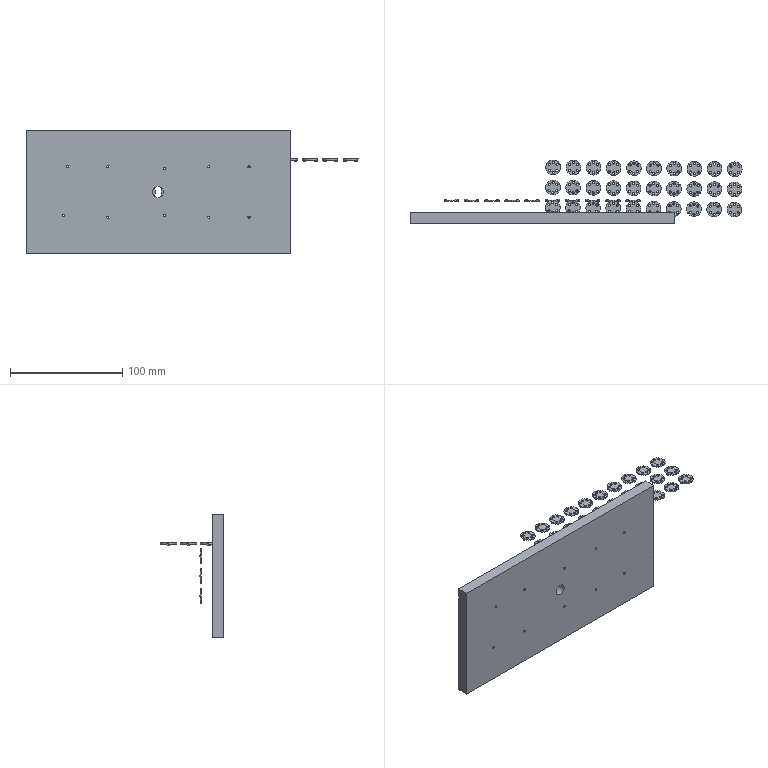NC program | NX | posted with a generic post | part box 296.27 x 56.878 x 110 mm
Lines 18830 to 20851 of 20851:
(DRILLING_COPY_1_COPY , TOOL : DJ-Ø3)
N37616 T04 M6
N37618 G17 G43 G0 G90 X84.467 Y15.117 Z1.5 B0. C0. S1500 H4 M3
N37620 G94 G81 G99 Z-2.1 F200. R0.
N37622 G0 Z4.
N37624 G81 X84.447 Y20.893 Z-2.1 R0.
N37626 G0 Z4.
N37628 G81 X81. Y22.5 Z-2.1 R0.
N37630 G0 Z4.
N37632 G81 X77.573 Y20.902 Z-2.1 R0.
N37634 G0 Z4.
N37636 G81 X77.553 Y15.107 Z-2.1 R0.
N37638 G0 Z4.
N37640 G81 X81. Y13.5 Z-2.1 R0.
N37642 G0 Z4.
N37644 G81 Y4.5 Z-2.1 R0.
N37646 G0 Z4.
N37648 G81 X77.573 Y2.902 Z-2.1 R0.
N37650 G0 Z4.
N37652 G81 X84.447 Y2.893 Z-2.1 R0.
N37654 G0 Z4.
N37656 G81 X84.467 Y-2.883 Z-2.1 R0.
N37658 G0 Z4.
N37660 G81 X81. Y-4.5 Z-2.1 R0.
N37662 G0 Z4.
N37664 G81 Y-13.5 Z-2.1 R0.
N37666 G0 Z4.
N37668 G81 X84.447 Y-15.107 Z-2.1 R0.
N37670 G0 Z4.
N37672 G81 X84.467 Y-20.883 Z-2.1 R0.
N37674 G0 Z4.
N37676 G81 X81. Y-22.5 Z-2.1 R0.
N37678 G0 Z4.
N37680 G81 X77.553 Y-20.893 Z-2.1 R0.
N37682 G0 Z4.
N37684 G81 X77.573 Y-15.098 Z-2.1 R0.
N37686 G0 Z4.
N37688 G81 X77.553 Y-2.893 Z-2.1 R0.
N37690 G0 Z4.
N37692 G81 X66.467 Y-2.883 Z-2.1 R0.
N37694 G0 Z4.
N37696 G81 X63. Y-4.5 Z-2.1 R0.
N37698 G0 Z4.
N37700 G81 X59.553 Y-2.893 Z-2.1 R0.
N37702 G0 Z4.
N37704 G81 X59.573 Y2.902 Z-2.1 R0.
N37706 G0 Z4.
N37708 G81 X66.447 Y2.893 Z-2.1 R0.
N37710 G0 Z4.
N37712 G81 X63. Y4.5 Z-2.1 R0.
N37714 G0 Z4.
N37716 G81 Y13.5 Z-2.1 R0.
N37718 G0 Z4.
N37720 G81 X66.467 Y15.117 Z-2.1 R0.
N37722 G0 Z4.
N37724 G81 X66.447 Y20.893 Z-2.1 R0.
N37726 G0 Z4.
N37728 G81 X63. Y22.5 Z-2.1 R0.
N37730 G0 Z4.
N37732 G81 X59.573 Y20.902 Z-2.1 R0.
N37734 G0 Z4.
N37736 G81 X59.553 Y15.107 Z-2.1 R0.
N37738 G0 Z4.
N37740 G81 X48.467 Y15.117 Z-2.1 R0.
N37742 G0 Z4.
N37744 G81 X48.447 Y20.893 Z-2.1 R0.
N37746 G0 Z4.
N37748 G81 X45. Y22.5 Z-2.1 R0.
N37750 G0 Z4.
N37752 G81 Y13.5 Z-2.1 R0.
N37754 G0 Z4.
N37756 G81 X41.553 Y15.107 Z-2.1 R0.
N37758 G0 Z4.
N37760 G81 X41.573 Y20.902 Z-2.1 R0.
N37762 G0 Z4.
N37764 G81 X30.447 Y20.893 Z-2.1 R0.
N37766 G0 Z4.
N37768 G81 X30.467 Y15.117 Z-2.1 R0.
N37770 G0 Z4.
N37772 G81 X23.553 Y15.107 Z-2.1 R0.
N37774 G0 Z4.
N37776 G81 X27. Y13.5 Z-2.1 R0.
N37778 G0 Z4.
N37780 G81 Y22.5 Z-2.1 R0.
N37782 G0 Z4.
N37784 G81 X23.573 Y20.902 Z-2.1 R0.
N37786 G0 Z4.
N37788 G81 X12.447 Y20.893 Z-2.1 R0.
N37790 G0 Z4.
N37792 G81 X9. Y22.5 Z-2.1 R0.
N37794 G0 Z4.
N37796 G81 X5.573 Y20.902 Z-2.1 R0.
N37798 G0 Z4.
N37800 G81 X5.553 Y15.107 Z-2.1 R0.
N37802 G0 Z4.
N37804 G81 X12.467 Y15.117 Z-2.1 R0.
N37806 G0 Z4.
N37808 G81 X9. Y13.5 Z-2.1 R0.
N37810 G0 Z4.
N37812 G81 Y4.5 Z-2.1 R0.
N37814 G0 Z4.
N37816 G81 X5.573 Y2.902 Z-2.1 R0.
N37818 G0 Z4.
N37820 G81 X5.553 Y-2.893 Z-2.1 R0.
N37822 G0 Z4.
N37824 G81 X9. Y-4.5 Z-2.1 R0.
N37826 G0 Z4.
N37828 G81 X12.467 Y-2.883 Z-2.1 R0.
N37830 G0 Z4.
N37832 G81 X12.447 Y2.893 Z-2.1 R0.
N37834 G0 Z4.
N37836 G81 X23.573 Y2.902 Z-2.1 R0.
N37838 G0 Z4.
N37840 G81 X23.553 Y-2.893 Z-2.1 R0.
N37842 G0 Z4.
N37844 G81 X27. Y-4.5 Z-2.1 R0.
N37846 G0 Z4.
N37848 G81 Y4.5 Z-2.1 R0.
N37850 G0 Z4.
N37852 G81 X30.447 Y2.893 Z-2.1 R0.
N37854 G0 Z4.
N37856 G81 X30.467 Y-2.883 Z-2.1 R0.
N37858 G0 Z4.
N37860 G81 X41.553 Y-2.893 Z-2.1 R0.
N37862 G0 Z4.
N37864 G81 X41.573 Y2.902 Z-2.1 R0.
N37866 G0 Z4.
N37868 G81 X45. Y4.5 Z-2.1 R0.
N37870 G0 Z4.
N37872 G81 X48.447 Y2.893 Z-2.1 R0.
N37874 G0 Z4.
N37876 G81 X48.467 Y-2.883 Z-2.1 R0.
N37878 G0 Z4.
N37880 G81 X45. Y-4.5 Z-2.1 R0.
N37882 G0 Z4.
N37884 G81 Y-13.5 Z-2.1 R0.
N37886 G0 Z4.
N37888 G81 X48.447 Y-15.107 Z-2.1 R0.
N37890 G0 Z4.
N37892 G81 X59.573 Y-15.098 Z-2.1 R0.
N37894 G0 Z4.
N37896 G81 X63. Y-13.5 Z-2.1 R0.
N37898 G0 Z4.
N37900 G81 X66.447 Y-15.107 Z-2.1 R0.
N37902 G0 Z4.
N37904 G81 X66.467 Y-20.883 Z-2.1 R0.
N37906 G0 Z4.
N37908 G81 X63. Y-22.5 Z-2.1 R0.
N37910 G0 Z4.
N37912 G81 X59.553 Y-20.893 Z-2.1 R0.
N37914 G0 Z4.
N37916 G81 X48.467 Y-20.883 Z-2.1 R0.
N37918 G0 Z4.
N37920 G81 X45. Y-22.5 Z-2.1 R0.
N37922 G0 Z4.
N37924 G81 X41.553 Y-20.893 Z-2.1 R0.
N37926 G0 Z4.
N37928 G81 X41.573 Y-15.098 Z-2.1 R0.
N37930 G0 Z4.
N37932 G81 X30.447 Y-15.107 Z-2.1 R0.
N37934 G0 Z4.
N37936 G81 X30.467 Y-20.883 Z-2.1 R0.
N37938 G0 Z4.
N37940 G81 X27. Y-22.5 Z-2.1 R0.
N37942 G0 Z4.
N37944 G81 X23.553 Y-20.893 Z-2.1 R0.
N37946 G0 Z4.
N37948 G81 X23.573 Y-15.098 Z-2.1 R0.
N37950 G0 Z4.
N37952 G81 X27. Y-13.5 Z-2.1 R0.
N37954 G0 Z4.
N37956 G81 X9. Z-2.1 R0.
N37958 G0 Z4.
N37960 G81 X12.447 Y-15.107 Z-2.1 R0.
N37962 G0 Z4.
N37964 G81 X12.467 Y-20.883 Z-2.1 R0.
N37966 G0 Z4.
N37968 G81 X9. Y-22.5 Z-2.1 R0.
N37970 G0 Z4.
N37972 G81 X5.553 Y-20.893 Z-2.1 R0.
N37974 G0 Z4.
N37976 G81 X5.573 Y-15.098 Z-2.1 R0.
N37978 G0 Z4.
N37980 G81 X-5.553 Y-15.107 Z-2.1 R0.
N37982 G0 Z4.
N37984 G81 X-5.533 Y-20.883 Z-2.1 R0.
N37986 G0 Z4.
N37988 G81 X-9. Y-22.5 Z-2.1 R0.
N37990 G0 Z4.
N37992 G81 X-12.447 Y-20.893 Z-2.1 R0.
N37994 G0 Z4.
N37996 G81 X-12.427 Y-15.098 Z-2.1 R0.
N37998 G0 Z4.
N38000 G81 X-9. Y-13.5 Z-2.1 R0.
N38002 G0 Z4.
N38004 G81 Y-4.5 Z-2.1 R0.
N38006 G0 Z4.
N38008 G81 X-12.447 Y-2.893 Z-2.1 R0.
N38010 G0 Z4.
N38012 G81 X-5.533 Y-2.883 Z-2.1 R0.
N38014 G0 Z4.
N38016 G81 X-5.553 Y2.893 Z-2.1 R0.
N38018 G0 Z4.
N38020 G81 X-9. Y4.5 Z-2.1 R0.
N38022 G0 Z4.
N38024 G81 X-12.427 Y2.902 Z-2.1 R0.
N38026 G0 Z4.
N38028 G81 X-12.447 Y15.107 Z-2.1 R0.
N38030 G0 Z4.
N38032 G81 X-9. Y13.5 Z-2.1 R0.
N38034 G0 Z4.
N38036 G81 X-5.533 Y15.117 Z-2.1 R0.
N38038 G0 Z4.
N38040 G81 X-5.553 Y20.893 Z-2.1 R0.
N38042 G0 Z4.
N38044 G81 X-9. Y22.5 Z-2.1 R0.
N38046 G0 Z4.
N38048 G81 X-12.427 Y20.902 Z-2.1 R0.
N38050 G0 Z4.
N38052 G81 X-23.553 Y20.893 Z-2.1 R0.
N38054 G0 Z4.
N38056 G81 X-23.533 Y15.117 Z-2.1 R0.
N38058 G0 Z4.
N38060 G81 X-27. Y13.5 Z-2.1 R0.
N38062 G0 Z4.
N38064 G81 Y22.5 Z-2.1 R0.
N38066 G0 Z4.
N38068 G81 X-30.427 Y20.902 Z-2.1 R0.
N38070 G0 Z4.
N38072 G81 X-30.447 Y15.107 Z-2.1 R0.
N38074 G0 Z4.
N38076 G81 X-41.533 Y15.117 Z-2.1 R0.
N38078 G0 Z4.
N38080 G81 X-41.553 Y20.893 Z-2.1 R0.
N38082 G0 Z4.
N38084 G81 X-45. Y22.5 Z-2.1 R0.
N38086 G0 Z4.
N38088 G81 X-48.427 Y20.902 Z-2.1 R0.
N38090 G0 Z4.
N38092 G81 X-48.447 Y15.107 Z-2.1 R0.
N38094 G0 Z4.
N38096 G81 X-45. Y13.5 Z-2.1 R0.
N38098 G0 Z4.
N38100 G81 Y4.5 Z-2.1 R0.
N38102 G0 Z4.
N38104 G81 X-41.553 Y2.893 Z-2.1 R0.
N38106 G0 Z4.
N38108 G81 X-41.533 Y-2.883 Z-2.1 R0.
N38110 G0 Z4.
N38112 G81 X-45. Y-4.5 Z-2.1 R0.
N38114 G0 Z4.
N38116 G81 X-48.447 Y-2.893 Z-2.1 R0.
N38118 G0 Z4.
N38120 G81 X-48.427 Y2.902 Z-2.1 R0.
N38122 G0 Z4.
N38124 G81 X-59.553 Y2.893 Z-2.1 R0.
N38126 G0 Z4.
N38128 G81 X-59.533 Y-2.883 Z-2.1 R0.
N38130 G0 Z4.
N38132 G81 X-63. Y-4.5 Z-2.1 R0.
N38134 G0 Z4.
N38136 G81 X-66.447 Y-2.893 Z-2.1 R0.
N38138 G0 Z4.
N38140 G81 X-66.427 Y2.902 Z-2.1 R0.
N38142 G0 Z4.
N38144 G81 X-63. Y4.5 Z-2.1 R0.
N38146 G0 Z4.
N38148 G81 Y13.5 Z-2.1 R0.
N38150 G0 Z4.
N38152 G81 X-59.533 Y15.117 Z-2.1 R0.
N38154 G0 Z4.
N38156 G81 X-59.553 Y20.893 Z-2.1 R0.
N38158 G0 Z4.
N38160 G81 X-63. Y22.5 Z-2.1 R0.
N38162 G0 Z4.
N38164 G81 X-66.427 Y20.902 Z-2.1 R0.
N38166 G0 Z4.
N38168 G81 X-66.447 Y15.107 Z-2.1 R0.
N38170 G0 Z4.
N38172 G81 X-77.533 Y15.117 Z-2.1 R0.
N38174 G0 Z4.
N38176 G81 X-77.553 Y20.893 Z-2.1 R0.
N38178 G0 Z4.
N38180 G81 X-81. Y22.5 Z-2.1 R0.
N38182 G0 Z4.
N38184 G81 X-84.427 Y20.902 Z-2.1 R0.
N38186 G0 Z4.
N38188 G81 X-84.447 Y15.107 Z-2.1 R0.
N38190 G0 Z4.
N38192 G81 X-81. Y13.5 Z-2.1 R0.
N38194 G0 Z4.
N38196 G81 Y4.5 Z-2.1 R0.
N38198 G0 Z4.
N38200 G81 X-77.553 Y2.893 Z-2.1 R0.
N38202 G0 Z4.
N38204 G81 X-84.427 Y2.902 Z-2.1 R0.
N38206 G0 Z4.
N38208 G81 X-84.447 Y-2.893 Z-2.1 R0.
N38210 G0 Z4.
N38212 G81 X-77.533 Y-2.883 Z-2.1 R0.
N38214 G0 Z4.
N38216 G81 X-81. Y-4.5 Z-2.1 R0.
N38218 G0 Z4.
N38220 G81 Y-13.5 Z-2.1 R0.
N38222 G0 Z4.
N38224 G81 X-77.553 Y-15.107 Z-2.1 R0.
N38226 G0 Z4.
N38228 G81 X-84.427 Y-15.098 Z-2.1 R0.
N38230 G0 Z4.
N38232 G81 X-84.447 Y-20.893 Z-2.1 R0.
N38234 G0 Z4.
N38236 G81 X-81. Y-22.5 Z-2.1 R0.
N38238 G0 Z4.
N38240 G81 X-77.533 Y-20.883 Z-2.1 R0.
N38242 G0 Z4.
N38244 G81 X-66.447 Y-20.893 Z-2.1 R0.
N38246 G0 Z4.
N38248 G81 X-66.427 Y-15.098 Z-2.1 R0.
N38250 G0 Z4.
N38252 G81 X-63. Y-13.5 Z-2.1 R0.
N38254 G0 Z4.
N38256 G81 Y-22.5 Z-2.1 R0.
N38258 G0 Z4.
N38260 G81 X-59.533 Y-20.883 Z-2.1 R0.
N38262 G0 Z4.
N38264 G81 X-59.553 Y-15.107 Z-2.1 R0.
N38266 G0 Z4.
N38268 G81 X-48.427 Y-15.098 Z-2.1 R0.
N38270 G0 Z4.
N38272 G81 X-48.447 Y-20.893 Z-2.1 R0.
N38274 G0 Z4.
N38276 G81 X-45. Y-22.5 Z-2.1 R0.
N38278 G0 Z4.
N38280 G81 Y-13.5 Z-2.1 R0.
N38282 G0 Z4.
N38284 G81 X-41.553 Y-15.107 Z-2.1 R0.
N38286 G0 Z4.
N38288 G81 X-41.533 Y-20.883 Z-2.1 R0.
N38290 G0 Z4.
N38292 G81 X-30.447 Y-20.893 Z-2.1 R0.
N38294 G0 Z4.
N38296 G81 X-27. Y-22.5 Z-2.1 R0.
N38298 G0 Z4.
N38300 G81 X-23.533 Y-20.883 Z-2.1 R0.
N38302 G0 Z4.
N38304 G81 X-23.553 Y-15.107 Z-2.1 R0.
N38306 G0 Z4.
N38308 G81 X-30.427 Y-15.098 Z-2.1 R0.
N38310 G0 Z4.
N38312 G81 X-27. Y-13.5 Z-2.1 R0.
N38314 G0 Z4.
N38316 G81 Y-4.5 Z-2.1 R0.
N38318 G0 Z4.
N38320 G81 X-30.447 Y-2.893 Z-2.1 R0.
N38322 G0 Z4.
N38324 G81 X-30.427 Y2.902 Z-2.1 R0.
N38326 G0 Z4.
N38328 G81 X-27. Y4.5 Z-2.1 R0.
N38330 G0 Z4.
N38332 G81 X-23.553 Y2.893 Z-2.1 R0.
N38334 G0 Z4.
N38336 G81 X-23.533 Y-2.883 Z-2.1 R0.
N38338 G0 Z4.
N38340 G80
N38342 G0 X-23.533 Y-2.883 Z1.5
(PLANAR_MILL_COPY_1_COPY , TOOL : DJ-Ø3)
N38344 X-75.902 Y-19.017 S5000
N38346 Z1.
N38348 G1 Z0.3 F5000.
N38350 Z-0.8 F800.
N38352 G41 X-76. Y-19. D4
N38354 X-77.75
N38356 Y-17.
N38358 X-74.25
N38360 Y-19.
N38362 X-76.
N38364 X-76.1
N38366 G40
N38368 X-76.198 Y-19.017
N38370 Z-0.5
N38372 G0 Z3.
N38374 X-85.902
N38376 G1 Z0.3 F5000.
N38378 Z-0.8 F800.
N38380 G41 X-86. Y-19.
N38382 X-87.75
N38384 Y-17.
N38386 X-84.25
N38388 Y-19.
N38390 X-86.
N38392 X-86.1
N38394 G40
N38396 X-86.198 Y-19.017
N38398 Z-0.5
N38400 G0 Z1.
(PLANAR_MILL_COPY_1_COPY_9_COPY , TOOL : DJ-Ø3)
N38402 Z1.
N38404 X-88.437 Y-15.352
N38406 G1 Z-1.8 F5000.
N38408 G41 X-88.454 Y-15.45 F800.
N38410 G3 X-87.954 Y-15.95 R0.5
N38412 G2 X-74.046 Y-15.95 R7.25
N38414 G3 X-73.546 Y-15.45 R0.5
N38416 G40
N38418 G1 X-73.563 Y-15.352
N38420 G0 Z2.
N38422 Y-20.648
N38424 G1 Z-1.8 F5000.
N38426 G41 X-73.546 Y-20.55 F800.
N38428 G3 X-74.046 Y-20.05 R0.5
N38430 G2 X-87.954 Y-20.05 R7.25
N38432 G3 X-88.454 Y-20.55 R0.5
N38434 G40
N38436 G1 X-88.437 Y-20.648
N38438 G0 Z1.
(PLANAR_MILL_COPY_1_COPY_12_COPY , TOOL : DJ-Ø3)
N38440 Z1.
N38442 X-75.902 Y-1.017
N38444 G1 Z0.3 F5000.
N38446 Z-0.8 F800.
N38448 G41 X-76. Y-1.
N38450 X-77.75
N38452 Y1.
N38454 X-74.25
N38456 Y-1.
N38458 X-76.
N38460 X-76.1
N38462 G40
N38464 X-76.198 Y-1.017
N38466 Z-0.5
N38468 G0 Z3.
N38470 X-85.902
N38472 G1 Z0.3 F5000.
N38474 Z-0.8 F800.
N38476 G41 X-86. Y-1.
N38478 X-87.75
N38480 Y1.
N38482 X-84.25
N38484 Y-1.
N38486 X-86.
N38488 X-86.1
N38490 G40
N38492 X-86.198 Y-1.017
N38494 Z-0.5
N38496 G0 Z1.
(PLANAR_MILL_COPY_1_COPY_9_COPY_1_COPY , TOOL : DJ-Ø3)
N38498 Z1.
N38500 X-88.437 Y2.648
N38502 G1 Z-1.8 F5000.
N38504 G41 X-88.454 Y2.55 F800.
N38506 G3 X-87.954 Y2.05 R0.5
N38508 G2 X-74.046 Y2.05 R7.25
N38510 G3 X-73.546 Y2.55 R0.5
N38512 G40
N38514 G1 X-73.563 Y2.648
N38516 G0 Z2.
N38518 Y-2.648
N38520 G1 Z-1.8 F5000.
N38522 G41 X-73.546 Y-2.55 F800.
N38524 G3 X-74.046 Y-2.05 R0.5
N38526 G2 X-87.954 Y-2.05 R7.25
N38528 G3 X-88.454 Y-2.55 R0.5
N38530 G40
N38532 G1 X-88.437 Y-2.648
N38534 G0 Z1.
(PLANAR_MILL_COPY_1_COPY_13_COPY , TOOL : DJ-Ø3)
N38536 Z1.
N38538 X-75.902 Y16.983
N38540 G1 Z0.3 F5000.
N38542 Z-0.8 F800.
N38544 G41 X-76. Y17.
N38546 X-77.75
N38548 Y19.
N38550 X-74.25
N38552 Y17.
N38554 X-76.
N38556 X-76.1
N38558 G40
N38560 X-76.198 Y16.983
N38562 Z-0.5
N38564 G0 Z3.
N38566 X-85.902
N38568 G1 Z0.3 F5000.
N38570 Z-0.8 F800.
N38572 G41 X-86. Y17.
N38574 X-87.75
N38576 Y19.
N38578 X-84.25
N38580 Y17.
N38582 X-86.
N38584 X-86.1
N38586 G40
N38588 X-86.198 Y16.983
N38590 Z-0.5
N38592 G0 Z1.
(PLANAR_MILL_COPY_1_COPY_9_COPY_2_COPY , TOOL : DJ-Ø3)
N38594 Z1.
N38596 X-88.437 Y20.648
N38598 G1 Z-1.8 F5000.
N38600 G41 X-88.454 Y20.55 F800.
N38602 G3 X-87.954 Y20.05 R0.5
N38604 G2 X-74.046 Y20.05 R7.25
N38606 G3 X-73.546 Y20.55 R0.5
N38608 G40
N38610 G1 X-73.563 Y20.648
N38612 G0 Z2.
N38614 Y15.352
N38616 G1 Z-1.8 F5000.
N38618 G41 X-73.546 Y15.45 F800.
N38620 G3 X-74.046 Y15.95 R0.5
N38622 G2 X-87.954 Y15.95 R7.25
N38624 G3 X-88.454 Y15.45 R0.5
N38626 G40
N38628 G1 X-88.437 Y15.352
N38630 G0 Z1.
(PLANAR_MILL_COPY_1_COPY_14_COPY , TOOL : DJ-Ø3)
N38632 Z1.
N38634 X-57.902 Y-19.017
N38636 G1 Z0.3 F5000.
N38638 Z-0.8 F800.
N38640 G41 X-58. Y-19.
N38642 X-59.75
N38644 Y-17.
N38646 X-56.25
N38648 Y-19.
N38650 X-58.
N38652 X-58.1
N38654 G40
N38656 X-58.198 Y-19.017
N38658 Z-0.5
N38660 G0 Z3.
N38662 X-67.902
N38664 G1 Z0.3 F5000.
N38666 Z-0.8 F800.
N38668 G41 X-68. Y-19.
N38670 X-69.75
N38672 Y-17.
N38674 X-66.25
N38676 Y-19.
N38678 X-68.
N38680 X-68.1
N38682 G40
N38684 X-68.198 Y-19.017
N38686 Z-0.5
N38688 G0 Z1.
(PLANAR_MILL_COPY_1_COPY_9_COPY_3_COPY , TOOL : DJ-Ø3)
N38690 Z1.
N38692 X-70.437 Y-15.352
N38694 G1 Z-1.8 F5000.
N38696 G41 X-70.454 Y-15.45 F800.
N38698 G3 X-69.954 Y-15.95 R0.5
N38700 G2 X-56.046 Y-15.95 R7.25
N38702 G3 X-55.546 Y-15.45 R0.5
N38704 G40
N38706 G1 X-55.563 Y-15.352
N38708 G0 Z2.
N38710 Y-20.648
N38712 G1 Z-1.8 F5000.
N38714 G41 X-55.546 Y-20.55 F800.
N38716 G3 X-56.046 Y-20.05 R0.5
N38718 G2 X-69.954 Y-20.05 R7.25
N38720 G3 X-70.454 Y-20.55 R0.5
N38722 G40
N38724 G1 X-70.437 Y-20.648
N38726 G0 Z1.
(PLANAR_MILL_COPY_1_COPY_15_COPY , TOOL : DJ-Ø3)
N38728 Z1.
N38730 X-57.902 Y-1.017
N38732 G1 Z0.3 F5000.
N38734 Z-0.8 F800.
N38736 G41 X-58. Y-1.
N38738 X-59.75
N38740 Y1.
N38742 X-56.25
N38744 Y-1.
N38746 X-58.
N38748 X-58.1
N38750 G40
N38752 X-58.198 Y-1.017
N38754 Z-0.5
N38756 G0 Z3.
N38758 X-67.902
N38760 G1 Z0.3 F5000.
N38762 Z-0.8 F800.
N38764 G41 X-68. Y-1.
N38766 X-69.75
N38768 Y1.
N38770 X-66.25
N38772 Y-1.
N38774 X-68.
N38776 X-68.1
N38778 G40
N38780 X-68.198 Y-1.017
N38782 Z-0.5
N38784 G0 Z1.
(PLANAR_MILL_COPY_1_COPY_9_COPY_4_COPY , TOOL : DJ-Ø3)
N38786 Z1.
N38788 X-70.437 Y2.648
N38790 G1 Z-1.8 F5000.
N38792 G41 X-70.454 Y2.55 F800.
N38794 G3 X-69.954 Y2.05 R0.5
N38796 G2 X-56.046 Y2.05 R7.25
N38798 G3 X-55.546 Y2.55 R0.5
N38800 G40
N38802 G1 X-55.563 Y2.648
N38804 G0 Z2.
N38806 Y-2.648
N38808 G1 Z-1.8 F5000.
N38810 G41 X-55.546 Y-2.55 F800.
N38812 G3 X-56.046 Y-2.05 R0.5
N38814 G2 X-69.954 Y-2.05 R7.25
N38816 G3 X-70.454 Y-2.55 R0.5
N38818 G40
N38820 G1 X-70.437 Y-2.648
N38822 G0 Z1.
(PLANAR_MILL_COPY_1_COPY_16_COPY , TOOL : DJ-Ø3)
N38824 Z1.
N38826 X-57.902 Y16.983
N38828 G1 Z0.3 F5000.
N38830 Z-0.8 F800.
N38832 G41 X-58. Y17.
N38834 X-59.75
N38836 Y19.
N38838 X-56.25
N38840 Y17.
N38842 X-58.
N38844 X-58.1
N38846 G40
N38848 X-58.198 Y16.983
N38850 Z-0.5
N38852 G0 Z3.
N38854 X-67.902
N38856 G1 Z0.3 F5000.
N38858 Z-0.8 F800.
N38860 G41 X-68. Y17.
N38862 X-69.75
N38864 Y19.
N38866 X-66.25
N38868 Y17.
N38870 X-68.
N38872 X-68.1
N38874 G40
N38876 X-68.198 Y16.983
N38878 Z-0.5
N38880 G0 Z1.
(PLANAR_MILL_COPY_1_COPY_9_COPY_5_COPY , TOOL : DJ-Ø3)
N38882 Z1.
N38884 X-70.437 Y20.648
N38886 G1 Z-1.8 F5000.
N38888 G41 X-70.454 Y20.55 F800.
N38890 G3 X-69.954 Y20.05 R0.5
N38892 G2 X-56.046 Y20.05 R7.25
N38894 G3 X-55.546 Y20.55 R0.5
N38896 G40
N38898 G1 X-55.563 Y20.648
N38900 G0 Z2.
N38902 Y15.352
N38904 G1 Z-1.8 F5000.
N38906 G41 X-55.546 Y15.45 F800.
N38908 G3 X-56.046 Y15.95 R0.5
N38910 G2 X-69.954 Y15.95 R7.25
N38912 G3 X-70.454 Y15.45 R0.5
N38914 G40
N38916 G1 X-70.437 Y15.352
N38918 G0 Z1.
(PLANAR_MILL_COPY_1_COPY_17_COPY , TOOL : DJ-Ø3)
N38920 Z1.
N38922 X-39.902 Y-19.017
N38924 G1 Z0.3 F5000.
N38926 Z-0.8 F800.
N38928 G41 X-40. Y-19.
N38930 X-41.75
N38932 Y-17.
N38934 X-38.25
N38936 Y-19.
N38938 X-40.
N38940 X-40.1
N38942 G40
N38944 X-40.198 Y-19.017
N38946 Z-0.5
N38948 G0 Z3.
N38950 X-49.902
N38952 G1 Z0.3 F5000.
N38954 Z-0.8 F800.
N38956 G41 X-50. Y-19.
N38958 X-51.75
N38960 Y-17.
N38962 X-48.25
N38964 Y-19.
N38966 X-50.
N38968 X-50.1
N38970 G40
N38972 X-50.198 Y-19.017
N38974 Z-0.5
N38976 G0 Z1.
(PLANAR_MILL_COPY_1_COPY_9_COPY_6_COPY , TOOL : DJ-Ø3)
N38978 Z1.
N38980 X-52.437 Y-15.352
N38982 G1 Z-1.8 F5000.
N38984 G41 X-52.454 Y-15.45 F800.
N38986 G3 X-51.954 Y-15.95 R0.5
N38988 G2 X-38.046 Y-15.95 R7.25
N38990 G3 X-37.546 Y-15.45 R0.5
N38992 G40
N38994 G1 X-37.563 Y-15.352
N38996 G0 Z2.
N38998 Y-20.648
N39000 G1 Z-1.8 F5000.
N39002 G41 X-37.546 Y-20.55 F800.
N39004 G3 X-38.046 Y-20.05 R0.5
N39006 G2 X-51.954 Y-20.05 R7.25
N39008 G3 X-52.454 Y-20.55 R0.5
N39010 G40
N39012 G1 X-52.437 Y-20.648
N39014 G0 Z1.
(PLANAR_MILL_COPY_1_COPY_18_COPY , TOOL : DJ-Ø3)
N39016 Z1.
N39018 X-39.902 Y-1.017
N39020 G1 Z0.3 F5000.
N39022 Z-0.8 F800.
N39024 G41 X-40. Y-1.
N39026 X-41.75
N39028 Y1.
N39030 X-38.25
N39032 Y-1.
N39034 X-40.
N39036 X-40.1
N39038 G40
N39040 X-40.198 Y-1.017
N39042 Z-0.5
N39044 G0 Z3.
N39046 X-49.902
N39048 G1 Z0.3 F5000.
N39050 Z-0.8 F800.
N39052 G41 X-50. Y-1.
N39054 X-51.75
N39056 Y1.
N39058 X-48.25
N39060 Y-1.
N39062 X-50.
N39064 X-50.1
N39066 G40
N39068 X-50.198 Y-1.017
N39070 Z-0.5
N39072 G0 Z1.
(PLANAR_MILL_COPY_1_COPY_9_COPY_7_COPY , TOOL : DJ-Ø3)
N39074 Z1.
N39076 X-52.437 Y2.648
N39078 G1 Z-1.8 F5000.
N39080 G41 X-52.454 Y2.55 F800.
N39082 G3 X-51.954 Y2.05 R0.5
N39084 G2 X-38.046 Y2.05 R7.25
N39086 G3 X-37.546 Y2.55 R0.5
N39088 G40
N39090 G1 X-37.563 Y2.648
N39092 G0 Z2.
N39094 Y-2.648
N39096 G1 Z-1.8 F5000.
N39098 G41 X-37.546 Y-2.55 F800.
N39100 G3 X-38.046 Y-2.05 R0.5
N39102 G2 X-51.954 Y-2.05 R7.25
N39104 G3 X-52.454 Y-2.55 R0.5
N39106 G40
N39108 G1 X-52.437 Y-2.648
N39110 G0 Z1.
(PLANAR_MILL_COPY_1_COPY_19_COPY , TOOL : DJ-Ø3)
N39112 Z1.
N39114 X-39.902 Y16.983
N39116 G1 Z0.3 F5000.
N39118 Z-0.8 F800.
N39120 G41 X-40. Y17.
N39122 X-41.75
N39124 Y19.
N39126 X-38.25
N39128 Y17.
N39130 X-40.
N39132 X-40.1
N39134 G40
N39136 X-40.198 Y16.983
N39138 Z-0.5
N39140 G0 Z3.
N39142 X-49.902
N39144 G1 Z0.3 F5000.
N39146 Z-0.8 F800.
N39148 G41 X-50. Y17.
N39150 X-51.75
N39152 Y19.
N39154 X-48.25
N39156 Y17.
N39158 X-50.
N39160 X-50.1
N39162 G40
N39164 X-50.198 Y16.983
N39166 Z-0.5
N39168 G0 Z1.
(PLANAR_MILL_COPY_1_COPY_9_COPY_8_COPY , TOOL : DJ-Ø3)
N39170 Z1.
N39172 X-52.437 Y20.648
N39174 G1 Z-1.8 F5000.
N39176 G41 X-52.454 Y20.55 F800.
N39178 G3 X-51.954 Y20.05 R0.5
N39180 G2 X-38.046 Y20.05 R7.25
N39182 G3 X-37.546 Y20.55 R0.5
N39184 G40
N39186 G1 X-37.563 Y20.648
N39188 G0 Z2.
N39190 Y15.352
N39192 G1 Z-1.8 F5000.
N39194 G41 X-37.546 Y15.45 F800.
N39196 G3 X-38.046 Y15.95 R0.5
N39198 G2 X-51.954 Y15.95 R7.25
N39200 G3 X-52.454 Y15.45 R0.5
N39202 G40
N39204 G1 X-52.437 Y15.352
N39206 G0 Z1.
(PLANAR_MILL_COPY_1_COPY_20_COPY , TOOL : DJ-Ø3)
N39208 Z1.
N39210 X-21.902 Y-19.017
N39212 G1 Z0.3 F5000.
N39214 Z-0.8 F800.
N39216 G41 X-22. Y-19.
N39218 X-23.75
N39220 Y-17.
N39222 X-20.25
N39224 Y-19.
N39226 X-22.
N39228 X-22.1
N39230 G40
N39232 X-22.198 Y-19.017
N39234 Z-0.5
N39236 G0 Z3.
N39238 X-31.902
N39240 G1 Z0.3 F5000.
N39242 Z-0.8 F800.
N39244 G41 X-32. Y-19.
N39246 X-33.75
N39248 Y-17.
N39250 X-30.25
N39252 Y-19.
N39254 X-32.
N39256 X-32.1
N39258 G40
N39260 X-32.198 Y-19.017
N39262 Z-0.5
N39264 G0 Z1.
(PLANAR_MILL_COPY_1_COPY_9_COPY_9_COPY , TOOL : DJ-Ø3)
N39266 Z1.
N39268 X-34.437 Y-15.352
N39270 G1 Z-1.8 F5000.
N39272 G41 X-34.454 Y-15.45 F800.
N39274 G3 X-33.954 Y-15.95 R0.5
N39276 G2 X-20.046 Y-15.95 R7.25
N39278 G3 X-19.546 Y-15.45 R0.5
N39280 G40
N39282 G1 X-19.563 Y-15.352
N39284 G0 Z2.
N39286 Y-20.648
N39288 G1 Z-1.8 F5000.
N39290 G41 X-19.546 Y-20.55 F800.
N39292 G3 X-20.046 Y-20.05 R0.5
N39294 G2 X-33.954 Y-20.05 R7.25
N39296 G3 X-34.454 Y-20.55 R0.5
N39298 G40
N39300 G1 X-34.437 Y-20.648
N39302 G0 Z1.
(PLANAR_MILL_COPY_1_COPY_21_COPY , TOOL : DJ-Ø3)
N39304 Z1.
N39306 X-21.902 Y-1.017
N39308 G1 Z0.3 F5000.
N39310 Z-0.8 F800.
N39312 G41 X-22. Y-1.
N39314 X-23.75
N39316 Y1.
N39318 X-20.25
N39320 Y-1.
N39322 X-22.
N39324 X-22.1
N39326 G40
N39328 X-22.198 Y-1.017
N39330 Z-0.5
N39332 G0 Z3.
N39334 X-31.902
N39336 G1 Z0.3 F5000.
N39338 Z-0.8 F800.
N39340 G41 X-32. Y-1.
N39342 X-33.75
N39344 Y1.
N39346 X-30.25
N39348 Y-1.
N39350 X-32.
N39352 X-32.1
N39354 G40
N39356 X-32.198 Y-1.017
N39358 Z-0.5
N39360 G0 Z1.
(PLANAR_MILL_COPY_1_COPY_9_COPY_10_COPY , TOOL : DJ-Ø3)
N39362 Z1.
N39364 X-34.437 Y2.648
N39366 G1 Z-1.8 F5000.
N39368 G41 X-34.454 Y2.55 F800.
N39370 G3 X-33.954 Y2.05 R0.5
N39372 G2 X-20.046 Y2.05 R7.25
N39374 G3 X-19.546 Y2.55 R0.5
N39376 G40
N39378 G1 X-19.563 Y2.648
N39380 G0 Z2.
N39382 Y-2.648
N39384 G1 Z-1.8 F5000.
N39386 G41 X-19.546 Y-2.55 F800.
N39388 G3 X-20.046 Y-2.05 R0.5
N39390 G2 X-33.954 Y-2.05 R7.25
N39392 G3 X-34.454 Y-2.55 R0.5
N39394 G40
N39396 G1 X-34.437 Y-2.648
N39398 G0 Z1.
(PLANAR_MILL_COPY_1_COPY_22_COPY , TOOL : DJ-Ø3)
N39400 Z1.
N39402 X-21.902 Y16.983
N39404 G1 Z0.3 F5000.
N39406 Z-0.8 F800.
N39408 G41 X-22. Y17.
N39410 X-23.75
N39412 Y19.
N39414 X-20.25
N39416 Y17.
N39418 X-22.
N39420 X-22.1
N39422 G40
N39424 X-22.198 Y16.983
N39426 Z-0.5
N39428 G0 Z3.
N39430 X-31.902
N39432 G1 Z0.3 F5000.
N39434 Z-0.8 F800.
N39436 G41 X-32. Y17.
N39438 X-33.75
N39440 Y19.
N39442 X-30.25
N39444 Y17.
N39446 X-32.
N39448 X-32.1
N39450 G40
N39452 X-32.198 Y16.983
N39454 Z-0.5
N39456 G0 Z1.
(PLANAR_MILL_COPY_1_COPY_9_COPY_11_COPY , TOOL : DJ-Ø3)
N39458 Z1.
N39460 X-34.437 Y20.648
N39462 G1 Z-1.8 F5000.
N39464 G41 X-34.454 Y20.55 F800.
N39466 G3 X-33.954 Y20.05 R0.5
N39468 G2 X-20.046 Y20.05 R7.25
N39470 G3 X-19.546 Y20.55 R0.5
N39472 G40
N39474 G1 X-19.563 Y20.648
N39476 G0 Z2.
N39478 Y15.352
N39480 G1 Z-1.8 F5000.
N39482 G41 X-19.546 Y15.45 F800.
N39484 G3 X-20.046 Y15.95 R0.5
N39486 G2 X-33.954 Y15.95 R7.25
N39488 G3 X-34.454 Y15.45 R0.5
N39490 G40
N39492 G1 X-34.437 Y15.352
N39494 G0 Z1.
(PLANAR_MILL_COPY_1_COPY_23_COPY , TOOL : DJ-Ø3)
N39496 Z1.
N39498 X-3.902 Y-19.017
N39500 G1 Z0.3 F5000.
N39502 Z-0.8 F800.
N39504 G41 X-4. Y-19.
N39506 X-5.75
N39508 Y-17.
N39510 X-2.25
N39512 Y-19.
N39514 X-4.
N39516 X-4.1
N39518 G40
N39520 X-4.198 Y-19.017
N39522 Z-0.5
N39524 G0 Z3.
N39526 X-13.902
N39528 G1 Z0.3 F5000.
N39530 Z-0.8 F800.
N39532 G41 X-14. Y-19.
N39534 X-15.75
N39536 Y-17.
N39538 X-12.25
N39540 Y-19.
N39542 X-14.
N39544 X-14.1
N39546 G40
N39548 X-14.198 Y-19.017
N39550 Z-0.5
N39552 G0 Z1.
(PLANAR_MILL_COPY_1_COPY_9_COPY_12_COPY , TOOL : DJ-Ø3)
N39554 Z1.
N39556 X-16.437 Y-15.352
N39558 G1 Z-1.8 F5000.
N39560 G41 X-16.454 Y-15.45 F800.
N39562 G3 X-15.954 Y-15.95 R0.5
N39564 G2 X-2.046 Y-15.95 R7.25
N39566 G3 X-1.546 Y-15.45 R0.5
N39568 G40
N39570 G1 X-1.563 Y-15.352
N39572 G0 Z2.
N39574 Y-20.648
N39576 G1 Z-1.8 F5000.
N39578 G41 X-1.546 Y-20.55 F800.
N39580 G3 X-2.046 Y-20.05 R0.5
N39582 G2 X-15.954 Y-20.05 R7.25
N39584 G3 X-16.454 Y-20.55 R0.5
N39586 G40
N39588 G1 X-16.437 Y-20.648
N39590 G0 Z1.
(PLANAR_MILL_COPY_1_COPY_24_COPY , TOOL : DJ-Ø3)
N39592 Z1.
N39594 X-3.902 Y-1.017
N39596 G1 Z0.3 F5000.
N39598 Z-0.8 F800.
N39600 G41 X-4. Y-1.
N39602 X-5.75
N39604 Y1.
N39606 X-2.25
N39608 Y-1.
N39610 X-4.
N39612 X-4.1
N39614 G40
N39616 X-4.198 Y-1.017
N39618 Z-0.5
N39620 G0 Z3.
N39622 X-13.902
N39624 G1 Z0.3 F5000.
N39626 Z-0.8 F800.
N39628 G41 X-14. Y-1.
N39630 X-15.75
N39632 Y1.
N39634 X-12.25
N39636 Y-1.
N39638 X-14.
N39640 X-14.1
N39642 G40
N39644 X-14.198 Y-1.017
N39646 Z-0.5
N39648 G0 Z1.
(PLANAR_MILL_COPY_1_COPY_9_COPY_13_COPY , TOOL : DJ-Ø3)
N39650 Z1.
N39652 X-16.437 Y2.648
N39654 G1 Z-1.8 F5000.
N39656 G41 X-16.454 Y2.55 F800.
N39658 G3 X-15.954 Y2.05 R0.5
N39660 G2 X-2.046 Y2.05 R7.25
N39662 G3 X-1.546 Y2.55 R0.5
N39664 G40
N39666 G1 X-1.563 Y2.648
N39668 G0 Z2.
N39670 Y-2.648
N39672 G1 Z-1.8 F5000.
N39674 G41 X-1.546 Y-2.55 F800.
N39676 G3 X-2.046 Y-2.05 R0.5
N39678 G2 X-15.954 Y-2.05 R7.25
N39680 G3 X-16.454 Y-2.55 R0.5
N39682 G40
N39684 G1 X-16.437 Y-2.648
N39686 G0 Z1.
(PLANAR_MILL_COPY_1_COPY_25_COPY , TOOL : DJ-Ø3)
N39688 Z1.
N39690 X-3.902 Y16.983
N39692 G1 Z0.3 F5000.
N39694 Z-0.8 F800.
N39696 G41 X-4. Y17.
N39698 X-5.75
N39700 Y19.
N39702 X-2.25
N39704 Y17.
N39706 X-4.
N39708 X-4.1
N39710 G40
N39712 X-4.198 Y16.983
N39714 Z-0.5
N39716 G0 Z3.
N39718 X-13.902
N39720 G1 Z0.3 F5000.
N39722 Z-0.8 F800.
N39724 G41 X-14. Y17.
N39726 X-15.75
N39728 Y19.
N39730 X-12.25
N39732 Y17.
N39734 X-14.
N39736 X-14.1
N39738 G40
N39740 X-14.198 Y16.983
N39742 Z-0.5
N39744 G0 Z1.
(PLANAR_MILL_COPY_1_COPY_9_COPY_14_COPY , TOOL : DJ-Ø3)
N39746 Z1.
N39748 X-16.437 Y20.648
N39750 G1 Z-1.8 F5000.
N39752 G41 X-16.454 Y20.55 F800.
N39754 G3 X-15.954 Y20.05 R0.5
N39756 G2 X-2.046 Y20.05 R7.25
N39758 G3 X-1.546 Y20.55 R0.5
N39760 G40
N39762 G1 X-1.563 Y20.648
N39764 G0 Z2.
N39766 Y15.352
N39768 G1 Z-1.8 F5000.
N39770 G41 X-1.546 Y15.45 F800.
N39772 G3 X-2.046 Y15.95 R0.5
N39774 G2 X-15.954 Y15.95 R7.25
N39776 G3 X-16.454 Y15.45 R0.5
N39778 G40
N39780 G1 X-16.437 Y15.352
N39782 G0 Z1.
(PLANAR_MILL_COPY_1_COPY_26_COPY , TOOL : DJ-Ø3)
N39784 Z1.
N39786 X14.098 Y-19.017
N39788 G1 Z0.3 F5000.
N39790 Z-0.8 F800.
N39792 G41 X14. Y-19.
N39794 X12.25
N39796 Y-17.
N39798 X15.75
N39800 Y-19.
N39802 X14.
N39804 X13.9
N39806 G40
N39808 X13.802 Y-19.017
N39810 Z-0.5
N39812 G0 Z3.
N39814 X4.098
N39816 G1 Z0.3 F5000.
N39818 Z-0.8 F800.
N39820 G41 X4. Y-19.
N39822 X2.25
N39824 Y-17.
N39826 X5.75
N39828 Y-19.
N39830 X4.
N39832 X3.9
N39834 G40
N39836 X3.802 Y-19.017
N39838 Z-0.5
N39840 G0 Z1.
(PLANAR_MILL_COPY_1_COPY_9_COPY_15_COPY , TOOL : DJ-Ø3)
N39842 Z1.
N39844 X1.563 Y-15.352
N39846 G1 Z-1.8 F5000.
N39848 G41 X1.546 Y-15.45 F800.
N39850 G3 X2.046 Y-15.95 R0.5
N39852 G2 X15.954 Y-15.95 R7.25
N39854 G3 X16.454 Y-15.45 R0.5
N39856 G40
N39858 G1 X16.437 Y-15.352
N39860 G0 Z2.
N39862 Y-20.648
N39864 G1 Z-1.8 F5000.
N39866 G41 X16.454 Y-20.55 F800.
N39868 G3 X15.954 Y-20.05 R0.5
N39870 G2 X2.046 Y-20.05 R7.25
N39872 G3 X1.546 Y-20.55 R0.5
N39874 G40
N39876 G1 X1.563 Y-20.648
N39878 G0 Z1.
(PLANAR_MILL_COPY_1_COPY_27_COPY , TOOL : DJ-Ø3)
N39880 Z1.
N39882 X14.098 Y-1.017
N39884 G1 Z0.3 F5000.
N39886 Z-0.8 F800.
N39888 G41 X14. Y-1.
N39890 X12.25
N39892 Y1.
N39894 X15.75
N39896 Y-1.
N39898 X14.
N39900 X13.9
N39902 G40
N39904 X13.802 Y-1.017
N39906 Z-0.5
N39908 G0 Z3.
N39910 X4.098
N39912 G1 Z0.3 F5000.
N39914 Z-0.8 F800.
N39916 G41 X4. Y-1.
N39918 X2.25
N39920 Y1.
N39922 X5.75
N39924 Y-1.
N39926 X4.
N39928 X3.9
N39930 G40
N39932 X3.802 Y-1.017
N39934 Z-0.5
N39936 G0 Z1.
(PLANAR_MILL_COPY_1_COPY_9_COPY_16_COPY , TOOL : DJ-Ø3)
N39938 Z1.
N39940 X1.563 Y2.648
N39942 G1 Z-1.8 F5000.
N39944 G41 X1.546 Y2.55 F800.
N39946 G3 X2.046 Y2.05 R0.5
N39948 G2 X15.954 Y2.05 R7.25
N39950 G3 X16.454 Y2.55 R0.5
N39952 G40
N39954 G1 X16.437 Y2.648
N39956 G0 Z2.
N39958 Y-2.648
N39960 G1 Z-1.8 F5000.
N39962 G41 X16.454 Y-2.55 F800.
N39964 G3 X15.954 Y-2.05 R0.5
N39966 G2 X2.046 Y-2.05 R7.25
N39968 G3 X1.546 Y-2.55 R0.5
N39970 G40
N39972 G1 X1.563 Y-2.648
N39974 G0 Z1.
(PLANAR_MILL_COPY_1_COPY_28_COPY , TOOL : DJ-Ø3)
N39976 Z1.
N39978 X14.098 Y16.983
N39980 G1 Z0.3 F5000.
N39982 Z-0.8 F800.
N39984 G41 X14. Y17.
N39986 X12.25
N39988 Y19.
N39990 X15.75
N39992 Y17.
N39994 X14.
N39996 X13.9
N39998 G40
N40000 X13.802 Y16.983
N40002 Z-0.5
N40004 G0 Z3.
N40006 X4.098
N40008 G1 Z0.3 F5000.
N40010 Z-0.8 F800.
N40012 G41 X4. Y17.
N40014 X2.25
N40016 Y19.
N40018 X5.75
N40020 Y17.
N40022 X4.
N40024 X3.9
N40026 G40
N40028 X3.802 Y16.983
N40030 Z-0.5
N40032 G0 Z1.
(PLANAR_MILL_COPY_1_COPY_9_COPY_17_COPY , TOOL : DJ-Ø3)
N40034 Z1.
N40036 X1.563 Y20.648
N40038 G1 Z-1.8 F5000.
N40040 G41 X1.546 Y20.55 F800.
N40042 G3 X2.046 Y20.05 R0.5
N40044 G2 X15.954 Y20.05 R7.25
N40046 G3 X16.454 Y20.55 R0.5
N40048 G40
N40050 G1 X16.437 Y20.648
N40052 G0 Z2.
N40054 Y15.352
N40056 G1 Z-1.8 F5000.
N40058 G41 X16.454 Y15.45 F800.
N40060 G3 X15.954 Y15.95 R0.5
N40062 G2 X2.046 Y15.95 R7.25
N40064 G3 X1.546 Y15.45 R0.5
N40066 G40
N40068 G1 X1.563 Y15.352
N40070 G0 Z1.
(PLANAR_MILL_COPY_1_COPY_29_COPY , TOOL : DJ-Ø3)
N40072 Z1.
N40074 X32.098 Y-19.017
N40076 G1 Z0.3 F5000.
N40078 Z-0.8 F800.
N40080 G41 X32. Y-19.
N40082 X30.25
N40084 Y-17.
N40086 X33.75
N40088 Y-19.
N40090 X32.
N40092 X31.9
N40094 G40
N40096 X31.802 Y-19.017
N40098 Z-0.5
N40100 G0 Z3.
N40102 X22.098
N40104 G1 Z0.3 F5000.
N40106 Z-0.8 F800.
N40108 G41 X22. Y-19.
N40110 X20.25
N40112 Y-17.
N40114 X23.75
N40116 Y-19.
N40118 X22.
N40120 X21.9
N40122 G40
N40124 X21.802 Y-19.017
N40126 Z-0.5
N40128 G0 Z1.
(PLANAR_MILL_COPY_1_COPY_9_COPY_18_COPY , TOOL : DJ-Ø3)
N40130 Z1.
N40132 X19.563 Y-15.352
N40134 G1 Z-1.8 F5000.
N40136 G41 X19.546 Y-15.45 F800.
N40138 G3 X20.046 Y-15.95 R0.5
N40140 G2 X33.954 Y-15.95 R7.25
N40142 G3 X34.454 Y-15.45 R0.5
N40144 G40
N40146 G1 X34.437 Y-15.352
N40148 G0 Z2.
N40150 Y-20.648
N40152 G1 Z-1.8 F5000.
N40154 G41 X34.454 Y-20.55 F800.
N40156 G3 X33.954 Y-20.05 R0.5
N40158 G2 X20.046 Y-20.05 R7.25
N40160 G3 X19.546 Y-20.55 R0.5
N40162 G40
N40164 G1 X19.563 Y-20.648
N40166 G0 Z1.
(PLANAR_MILL_COPY_1_COPY_30_COPY , TOOL : DJ-Ø3)
N40168 Z1.
N40170 X32.098 Y-1.017
N40172 G1 Z0.3 F5000.
N40174 Z-0.8 F800.
N40176 G41 X32. Y-1.
N40178 X30.25
N40180 Y1.
N40182 X33.75
N40184 Y-1.
N40186 X32.
N40188 X31.9
N40190 G40
N40192 X31.802 Y-1.017
N40194 Z-0.5
N40196 G0 Z3.
N40198 X22.098
N40200 G1 Z0.3 F5000.
N40202 Z-0.8 F800.
N40204 G41 X22. Y-1.
N40206 X20.25
N40208 Y1.
N40210 X23.75
N40212 Y-1.
N40214 X22.
N40216 X21.9
N40218 G40
N40220 X21.802 Y-1.017
N40222 Z-0.5
N40224 G0 Z1.
(PLANAR_MILL_COPY_1_COPY_9_COPY_19_COPY , TOOL : DJ-Ø3)
N40226 Z1.
N40228 X19.563 Y2.648
N40230 G1 Z-1.8 F5000.
N40232 G41 X19.546 Y2.55 F800.
N40234 G3 X20.046 Y2.05 R0.5
N40236 G2 X33.954 Y2.05 R7.25
N40238 G3 X34.454 Y2.55 R0.5
N40240 G40
N40242 G1 X34.437 Y2.648
N40244 G0 Z2.
N40246 Y-2.648
N40248 G1 Z-1.8 F5000.
N40250 G41 X34.454 Y-2.55 F800.
N40252 G3 X33.954 Y-2.05 R0.5
N40254 G2 X20.046 Y-2.05 R7.25
N40256 G3 X19.546 Y-2.55 R0.5
N40258 G40
N40260 G1 X19.563 Y-2.648
N40262 G0 Z1.
(PLANAR_MILL_COPY_1_COPY_31_COPY , TOOL : DJ-Ø3)
N40264 Z1.
N40266 X32.098 Y16.983
N40268 G1 Z0.3 F5000.
N40270 Z-0.8 F800.
N40272 G41 X32. Y17.
N40274 X30.25
N40276 Y19.
N40278 X33.75
N40280 Y17.
N40282 X32.
N40284 X31.9
N40286 G40
N40288 X31.802 Y16.983
N40290 Z-0.5
N40292 G0 Z3.
N40294 X22.098
N40296 G1 Z0.3 F5000.
N40298 Z-0.8 F800.
N40300 G41 X22. Y17.
N40302 X20.25
N40304 Y19.
N40306 X23.75
N40308 Y17.
N40310 X22.
N40312 X21.9
N40314 G40
N40316 X21.802 Y16.983
N40318 Z-0.5
N40320 G0 Z1.
(PLANAR_MILL_COPY_1_COPY_9_COPY_20_COPY , TOOL : DJ-Ø3)
N40322 Z1.
N40324 X19.563 Y20.648
N40326 G1 Z-1.8 F5000.
N40328 G41 X19.546 Y20.55 F800.
N40330 G3 X20.046 Y20.05 R0.5
N40332 G2 X33.954 Y20.05 R7.25
N40334 G3 X34.454 Y20.55 R0.5
N40336 G40
N40338 G1 X34.437 Y20.648
N40340 G0 Z2.
N40342 Y15.352
N40344 G1 Z-1.8 F5000.
N40346 G41 X34.454 Y15.45 F800.
N40348 G3 X33.954 Y15.95 R0.5
N40350 G2 X20.046 Y15.95 R7.25
N40352 G3 X19.546 Y15.45 R0.5
N40354 G40
N40356 G1 X19.563 Y15.352
N40358 G0 Z1.
(PLANAR_MILL_COPY_1_COPY_32_COPY , TOOL : DJ-Ø3)
N40360 Z1.
N40362 X50.098 Y-19.017
N40364 G1 Z0.3 F5000.
N40366 Z-0.8 F800.
N40368 G41 X50. Y-19.
N40370 X48.25
N40372 Y-17.
N40374 X51.75
N40376 Y-19.
N40378 X50.
N40380 X49.9
N40382 G40
N40384 X49.802 Y-19.017
N40386 Z-0.5
N40388 G0 Z3.
N40390 X40.098
N40392 G1 Z0.3 F5000.
N40394 Z-0.8 F800.
N40396 G41 X40. Y-19.
N40398 X38.25
N40400 Y-17.
N40402 X41.75
N40404 Y-19.
N40406 X40.
N40408 X39.9
N40410 G40
N40412 X39.802 Y-19.017
N40414 Z-0.5
N40416 G0 Z1.
(PLANAR_MILL_COPY_1_COPY_9_COPY_21_COPY , TOOL : DJ-Ø3)
N40418 Z1.
N40420 X37.563 Y-15.352
N40422 G1 Z-1.8 F5000.
N40424 G41 X37.546 Y-15.45 F800.
N40426 G3 X38.046 Y-15.95 R0.5
N40428 G2 X51.954 Y-15.95 R7.25
N40430 G3 X52.454 Y-15.45 R0.5
N40432 G40
N40434 G1 X52.437 Y-15.352
N40436 G0 Z2.
N40438 Y-20.648
N40440 G1 Z-1.8 F5000.
N40442 G41 X52.454 Y-20.55 F800.
N40444 G3 X51.954 Y-20.05 R0.5
N40446 G2 X38.046 Y-20.05 R7.25
N40448 G3 X37.546 Y-20.55 R0.5
N40450 G40
N40452 G1 X37.563 Y-20.648
N40454 G0 Z1.
(PLANAR_MILL_COPY_1_COPY_33_COPY , TOOL : DJ-Ø3)
N40456 Z1.
N40458 X50.098 Y-1.017
N40460 G1 Z0.3 F5000.
N40462 Z-0.8 F800.
N40464 G41 X50. Y-1.
N40466 X48.25
N40468 Y1.
N40470 X51.75
N40472 Y-1.
N40474 X50.
N40476 X49.9
N40478 G40
N40480 X49.802 Y-1.017
N40482 Z-0.5
N40484 G0 Z3.
N40486 X40.098
N40488 G1 Z0.3 F5000.
N40490 Z-0.8 F800.
N40492 G41 X40. Y-1.
N40494 X38.25
N40496 Y1.
N40498 X41.75
N40500 Y-1.
N40502 X40.
N40504 X39.9
N40506 G40
N40508 X39.802 Y-1.017
N40510 Z-0.5
N40512 G0 Z1.
(PLANAR_MILL_COPY_1_COPY_9_COPY_22_COPY , TOOL : DJ-Ø3)
N40514 Z1.
N40516 X37.563 Y2.648
N40518 G1 Z-1.8 F5000.
N40520 G41 X37.546 Y2.55 F800.
N40522 G3 X38.046 Y2.05 R0.5
N40524 G2 X51.954 Y2.05 R7.25
N40526 G3 X52.454 Y2.55 R0.5
N40528 G40
N40530 G1 X52.437 Y2.648
N40532 G0 Z2.
N40534 Y-2.648
N40536 G1 Z-1.8 F5000.
N40538 G41 X52.454 Y-2.55 F800.
N40540 G3 X51.954 Y-2.05 R0.5
N40542 G2 X38.046 Y-2.05 R7.25
N40544 G3 X37.546 Y-2.55 R0.5
N40546 G40
N40548 G1 X37.563 Y-2.648
N40550 G0 Z1.
(PLANAR_MILL_COPY_1_COPY_34_COPY , TOOL : DJ-Ø3)
N40552 Z1.
N40554 X50.098 Y16.983
N40556 G1 Z0.3 F5000.
N40558 Z-0.8 F800.
N40560 G41 X50. Y17.
N40562 X48.25
N40564 Y19.
N40566 X51.75
N40568 Y17.
N40570 X50.
N40572 X49.9
N40574 G40
N40576 X49.802 Y16.983
N40578 Z-0.5
N40580 G0 Z3.
N40582 X40.098
N40584 G1 Z0.3 F5000.
N40586 Z-0.8 F800.
N40588 G41 X40. Y17.
N40590 X38.25
N40592 Y19.
N40594 X41.75
N40596 Y17.
N40598 X40.
N40600 X39.9
N40602 G40
N40604 X39.802 Y16.983
N40606 Z-0.5
N40608 G0 Z1.
(PLANAR_MILL_COPY_1_COPY_9_COPY_23_COPY , TOOL : DJ-Ø3)
N40610 Z1.
N40612 X37.563 Y20.648
N40614 G1 Z-1.8 F5000.
N40616 G41 X37.546 Y20.55 F800.
N40618 G3 X38.046 Y20.05 R0.5
N40620 G2 X51.954 Y20.05 R7.25
N40622 G3 X52.454 Y20.55 R0.5
N40624 G40
N40626 G1 X52.437 Y20.648
N40628 G0 Z2.
N40630 Y15.352
N40632 G1 Z-1.8 F5000.
N40634 G41 X52.454 Y15.45 F800.
N40636 G3 X51.954 Y15.95 R0.5
N40638 G2 X38.046 Y15.95 R7.25
N40640 G3 X37.546 Y15.45 R0.5
N40642 G40
N40644 G1 X37.563 Y15.352
N40646 G0 Z1.
(PLANAR_MILL_COPY_1_COPY_35_COPY , TOOL : DJ-Ø3)
N40648 Z1.
N40650 X68.098 Y-19.017
N40652 G1 Z0.3 F5000.
N40654 Z-0.8 F800.
N40656 G41 X68. Y-19.
N40658 X66.25
N40660 Y-17.
N40662 X69.75
N40664 Y-19.
N40666 X68.
N40668 X67.9
N40670 G40
N40672 X67.802 Y-19.017
N40674 Z-0.5
N40676 G0 Z3.
N40678 X58.098
N40680 G1 Z0.3 F5000.
N40682 Z-0.8 F800.
N40684 G41 X58. Y-19.
N40686 X56.25
N40688 Y-17.
N40690 X59.75
N40692 Y-19.
N40694 X58.
N40696 X57.9
N40698 G40
N40700 X57.802 Y-19.017
N40702 Z-0.5
N40704 G0 Z1.
(PLANAR_MILL_COPY_1_COPY_9_COPY_24_COPY , TOOL : DJ-Ø3)
N40706 Z1.
N40708 X55.563 Y-15.352
N40710 G1 Z-1.8 F5000.
N40712 G41 X55.546 Y-15.45 F800.
N40714 G3 X56.046 Y-15.95 R0.5
N40716 G2 X69.954 Y-15.95 R7.25
N40718 G3 X70.454 Y-15.45 R0.5
N40720 G40
N40722 G1 X70.437 Y-15.352
N40724 G0 Z2.
N40726 Y-20.648
N40728 G1 Z-1.8 F5000.
N40730 G41 X70.454 Y-20.55 F800.
N40732 G3 X69.954 Y-20.05 R0.5
N40734 G2 X56.046 Y-20.05 R7.25
N40736 G3 X55.546 Y-20.55 R0.5
N40738 G40
N40740 G1 X55.563 Y-20.648
N40742 G0 Z1.
(PLANAR_MILL_COPY_1_COPY_36_COPY , TOOL : DJ-Ø3)
N40744 Z1.
N40746 X68.098 Y-1.017
N40748 G1 Z0.3 F5000.
N40750 Z-0.8 F800.
N40752 G41 X68. Y-1.
N40754 X66.25
N40756 Y1.
N40758 X69.75
N40760 Y-1.
N40762 X68.
N40764 X67.9
N40766 G40
N40768 X67.802 Y-1.017
N40770 Z-0.5
N40772 G0 Z3.
N40774 X58.098
N40776 G1 Z0.3 F5000.
N40778 Z-0.8 F800.
N40780 G41 X58. Y-1.
N40782 X56.25
N40784 Y1.
N40786 X59.75
N40788 Y-1.
N40790 X58.
N40792 X57.9
N40794 G40
N40796 X57.802 Y-1.017
N40798 Z-0.5
N40800 G0 Z1.
(PLANAR_MILL_COPY_1_COPY_9_COPY_25_COPY , TOOL : DJ-Ø3)
N40802 Z1.
N40804 X55.563 Y2.648
N40806 G1 Z-1.8 F5000.
N40808 G41 X55.546 Y2.55 F800.
N40810 G3 X56.046 Y2.05 R0.5
N40812 G2 X69.954 Y2.05 R7.25
N40814 G3 X70.454 Y2.55 R0.5
N40816 G40
N40818 G1 X70.437 Y2.648
N40820 G0 Z2.
N40822 Y-2.648
N40824 G1 Z-1.8 F5000.
N40826 G41 X70.454 Y-2.55 F800.
N40828 G3 X69.954 Y-2.05 R0.5
N40830 G2 X56.046 Y-2.05 R7.25
N40832 G3 X55.546 Y-2.55 R0.5
N40834 G40
N40836 G1 X55.563 Y-2.648
N40838 G0 Z1.
(PLANAR_MILL_COPY_1_COPY_37_COPY , TOOL : DJ-Ø3)
N40840 Z1.
N40842 X68.098 Y16.983
N40844 G1 Z0.3 F5000.
N40846 Z-0.8 F800.
N40848 G41 X68. Y17.
N40850 X66.25
N40852 Y19.
N40854 X69.75
N40856 Y17.
N40858 X68.
N40860 X67.9
N40862 G40
N40864 X67.802 Y16.983
N40866 Z-0.5
N40868 G0 Z3.
N40870 X58.098
N40872 G1 Z0.3 F5000.
N40874 Z-0.8 F800.
N40876 G41 X58. Y17.
N40878 X56.25
N40880 Y19.
N40882 X59.75
N40884 Y17.
N40886 X58.
N40888 X57.9
N40890 G40
N40892 X57.802 Y16.983
N40894 Z-0.5
N40896 G0 Z1.
(PLANAR_MILL_COPY_1_COPY_9_COPY_26_COPY , TOOL : DJ-Ø3)
N40898 Z1.
N40900 X55.563 Y20.648
N40902 G1 Z-1.8 F5000.
N40904 G41 X55.546 Y20.55 F800.
N40906 G3 X56.046 Y20.05 R0.5
N40908 G2 X69.954 Y20.05 R7.25
N40910 G3 X70.454 Y20.55 R0.5
N40912 G40
N40914 G1 X70.437 Y20.648
N40916 G0 Z2.
N40918 Y15.352
N40920 G1 Z-1.8 F5000.
N40922 G41 X70.454 Y15.45 F800.
N40924 G3 X69.954 Y15.95 R0.5
N40926 G2 X56.046 Y15.95 R7.25
N40928 G3 X55.546 Y15.45 R0.5
N40930 G40
N40932 G1 X55.563 Y15.352
N40934 G0 Z1.
(PLANAR_MILL_COPY_1_COPY_38_COPY , TOOL : DJ-Ø3)
N40936 Z1.
N40938 X86.098 Y-19.017
N40940 G1 Z0.3 F5000.
N40942 Z-0.8 F800.
N40944 G41 X86. Y-19.
N40946 X84.25
N40948 Y-17.
N40950 X87.75
N40952 Y-19.
N40954 X86.
N40956 X85.9
N40958 G40
N40960 X85.802 Y-19.017
N40962 Z-0.5
N40964 G0 Z3.
N40966 X76.098
N40968 G1 Z0.3 F5000.
N40970 Z-0.8 F800.
N40972 G41 X76. Y-19.
N40974 X74.25
N40976 Y-17.
N40978 X77.75
N40980 Y-19.
N40982 X76.
N40984 X75.9
N40986 G40
N40988 X75.802 Y-19.017
N40990 Z-0.5
N40992 G0 Z1.
(PLANAR_MILL_COPY_1_COPY_9_COPY_27_COPY , TOOL : DJ-Ø3)
N40994 Z1.
N40996 X73.563 Y-15.352
N40998 G1 Z-1.8 F5000.
N41000 G41 X73.546 Y-15.45 F800.
N41002 G3 X74.046 Y-15.95 R0.5
N41004 G2 X87.954 Y-15.95 R7.25
N41006 G3 X88.454 Y-15.45 R0.5
N41008 G40
N41010 G1 X88.437 Y-15.352
N41012 G0 Z2.
N41014 Y-20.648
N41016 G1 Z-1.8 F5000.
N41018 G41 X88.454 Y-20.55 F800.
N41020 G3 X87.954 Y-20.05 R0.5
N41022 G2 X74.046 Y-20.05 R7.25
N41024 G3 X73.546 Y-20.55 R0.5
N41026 G40
N41028 G1 X73.563 Y-20.648
N41030 G0 Z1.
(PLANAR_MILL_COPY_1_COPY_39_COPY , TOOL : DJ-Ø3)
N41032 Z1.
N41034 X86.098 Y-1.017
N41036 G1 Z0.3 F5000.
N41038 Z-0.8 F800.
N41040 G41 X86. Y-1.
N41042 X84.25
N41044 Y1.
N41046 X87.75
N41048 Y-1.
N41050 X86.
N41052 X85.9
N41054 G40
N41056 X85.802 Y-1.017
N41058 Z-0.5
N41060 G0 Z3.
N41062 X76.098
N41064 G1 Z0.3 F5000.
N41066 Z-0.8 F800.
N41068 G41 X76. Y-1.
N41070 X74.25
N41072 Y1.
N41074 X77.75
N41076 Y-1.
N41078 X76.
N41080 X75.9
N41082 G40
N41084 X75.802 Y-1.017
N41086 Z-0.5
N41088 G0 Z1.
(PLANAR_MILL_COPY_1_COPY_9_COPY_28_COPY , TOOL : DJ-Ø3)
N41090 Z1.
N41092 X73.563 Y2.648
N41094 G1 Z-1.8 F5000.
N41096 G41 X73.546 Y2.55 F800.
N41098 G3 X74.046 Y2.05 R0.5
N41100 G2 X87.954 Y2.05 R7.25
N41102 G3 X88.454 Y2.55 R0.5
N41104 G40
N41106 G1 X88.437 Y2.648
N41108 G0 Z2.
N41110 Y-2.648
N41112 G1 Z-1.8 F5000.
N41114 G41 X88.454 Y-2.55 F800.
N41116 G3 X87.954 Y-2.05 R0.5
N41118 G2 X74.046 Y-2.05 R7.25
N41120 G3 X73.546 Y-2.55 R0.5
N41122 G40
N41124 G1 X73.563 Y-2.648
N41126 G0 Z1.
(PLANAR_MILL_COPY_1_COPY_40_COPY , TOOL : DJ-Ø3)
N41128 Z1.
N41130 X86.098 Y16.983
N41132 G1 Z0.3 F5000.
N41134 Z-0.8 F800.
N41136 G41 X86. Y17.
N41138 X84.25
N41140 Y19.
N41142 X87.75
N41144 Y17.
N41146 X86.
N41148 X85.9
N41150 G40
N41152 X85.802 Y16.983
N41154 Z-0.5
N41156 G0 Z3.
N41158 X76.098
N41160 G1 Z0.3 F5000.
N41162 Z-0.8 F800.
N41164 G41 X76. Y17.
N41166 X74.25
N41168 Y19.
N41170 X77.75
N41172 Y17.
N41174 X76.
N41176 X75.9
N41178 G40
N41180 X75.802 Y16.983
N41182 Z-0.5
N41184 G0 Z1.
(PLANAR_MILL_COPY_1_COPY_9_COPY_29_COPY , TOOL : DJ-Ø3)
N41186 Z1.
N41188 X73.563 Y20.648
N41190 G1 Z-1.8 F5000.
N41192 G41 X73.546 Y20.55 F800.
N41194 G3 X74.046 Y20.05 R0.5
N41196 G2 X87.954 Y20.05 R7.25
N41198 G3 X88.454 Y20.55 R0.5
N41200 G40
N41202 G1 X88.437 Y20.648
N41204 G0 Z2.
N41206 Y15.352
N41208 G1 Z-1.8 F5000.
N41210 G41 X88.454 Y15.45 F800.
N41212 G3 X87.954 Y15.95 R0.5
N41214 G2 X74.046 Y15.95 R7.25
N41216 G3 X73.546 Y15.45 R0.5
N41218 G40
N41220 G1 X73.563 Y15.352
N41222 G0 Z1.
N41224 M5
(FLOOR_WALL , TOOL : D16)
N41226 T15 M6
N41228 G54
N41230 G17 G0 G90 X129. Y-51. B0. C0. S4000 M3
N41232 G43 Z50. H15
N41234 Z3. B-180.
N41236 G94 G1 Z0. F1000.
N41238 X126.
N41240 X-126.
N41242 Y-39.933
N41244 X126.
N41246 Y-28.866
N41248 X-126.
N41250 Y-17.8
N41252 X126.
N41254 Y-6.733
N41256 X-126.
N41258 Y4.333
N41260 X126.
N41262 Y15.4
N41264 X-126.
N41266 Y26.466
N41268 X126.
N41270 Y37.533
N41272 X-126.
N41274 Y48.6
N41276 X126.
N41278 X129.
N41280 Z3.
N41282 G0 Z50.
N41284 M5
N41286 M2